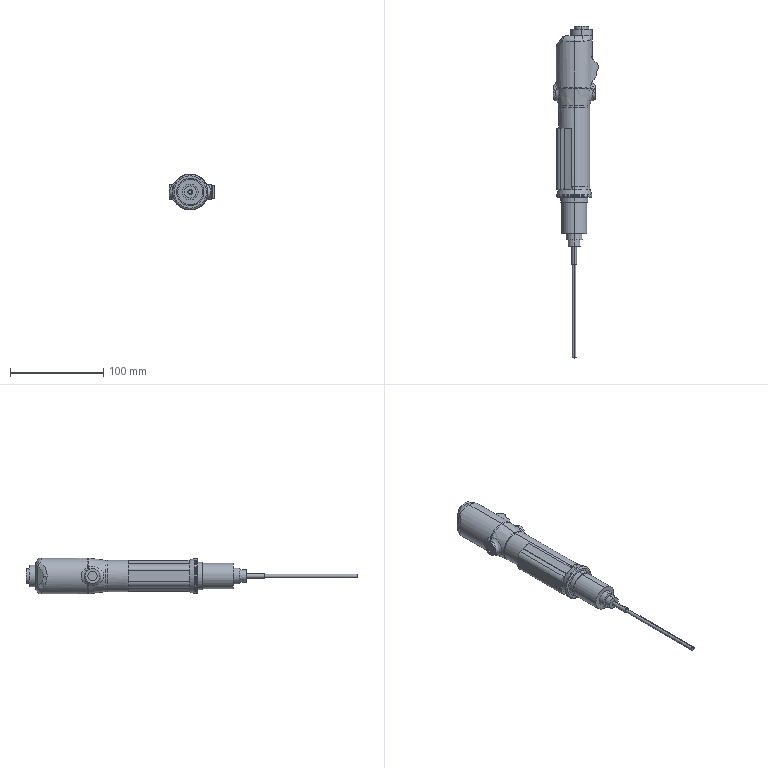Part | NX | 1 solid | 108 faces | box 48.781 x 356.5 x 38.5 mm | volume 209713 mm3 | cylinder 37 | plane 31 | spline 20 | torus 14 | cone 4 | sphere 2 | commonest cylinder face diameters 15.5 x6 10 x4 12 x3 4 x2 5 x2 13 x2